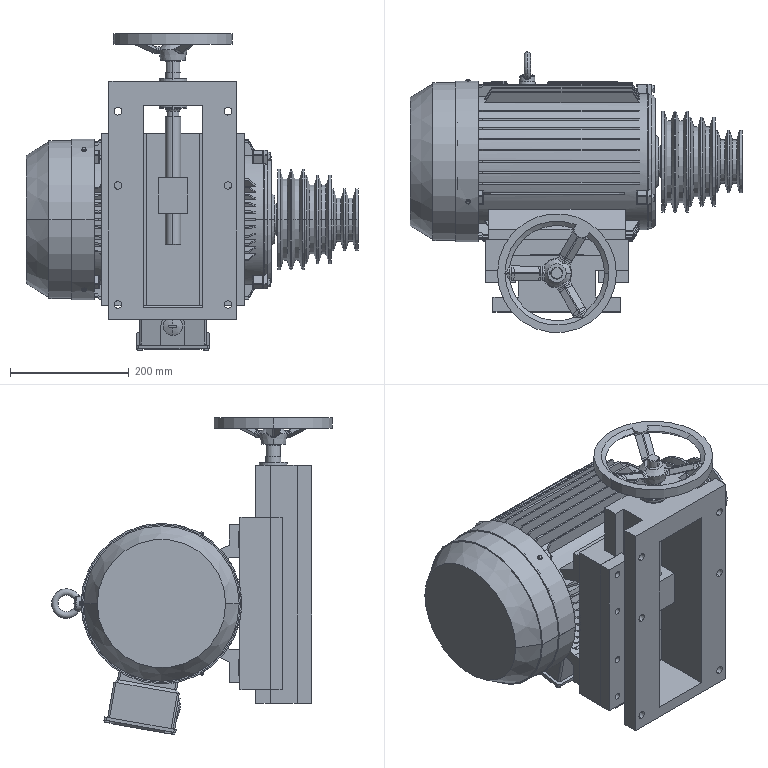Part | SolidWorks | features ReferencePattern 2, LocalLPattern 1, MirrorCompFeat 1 | 24 solids | 1639 faces | box 558.147 x 472.8 x 532.819 mm | volume 28170554 mm3 | plane 807 | cylinder 372 | cone 252 | torus 110 | sphere 90 | spline 8 | commonest cylinder face diameters 2 x69 6 x35 8.5 x20 11 x16 12 x16 6.701 x12